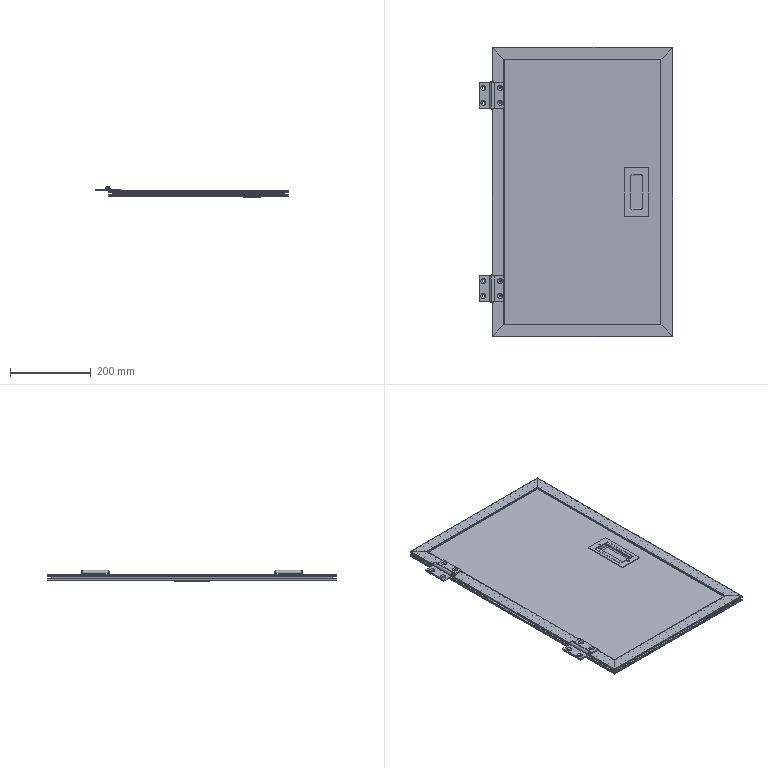Part | SolidWorks | features MoveCopyBody 3, Stock 3, ICE 2, HoleWzd 1, WeldMemberFeat 1, WeldmentFeature 1 | 8 solids | 320 faces | box 479 x 716 x 28.7 mm | volume 2209048 mm3 | plane 165 | cylinder 111 | cone 36 | sphere 8 | commonest cylinder face diameters 5 x28 2 x20 10 x16 4 x12 15 x11 6.4 x8